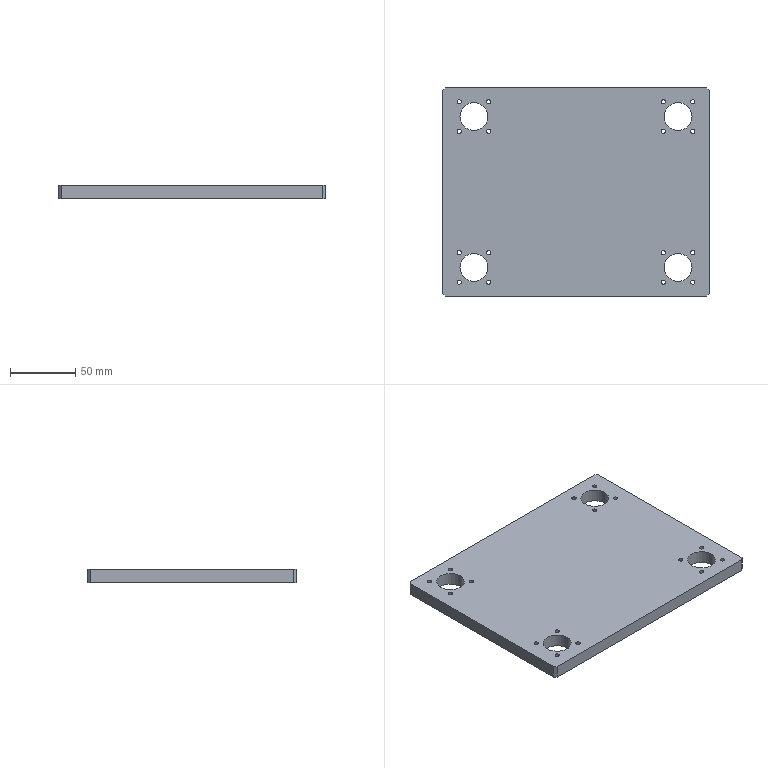Part | SolidWorks | features Chamfer 1, Cut 1, Extrusion 1, HoleWzd 1 | 1 solid | 50 faces | box 205 x 160 x 10 mm | volume 312030 mm3 | cylinder 40 | plane 10 | commonest cylinder face diameters 3.3 x32 21.5 x8